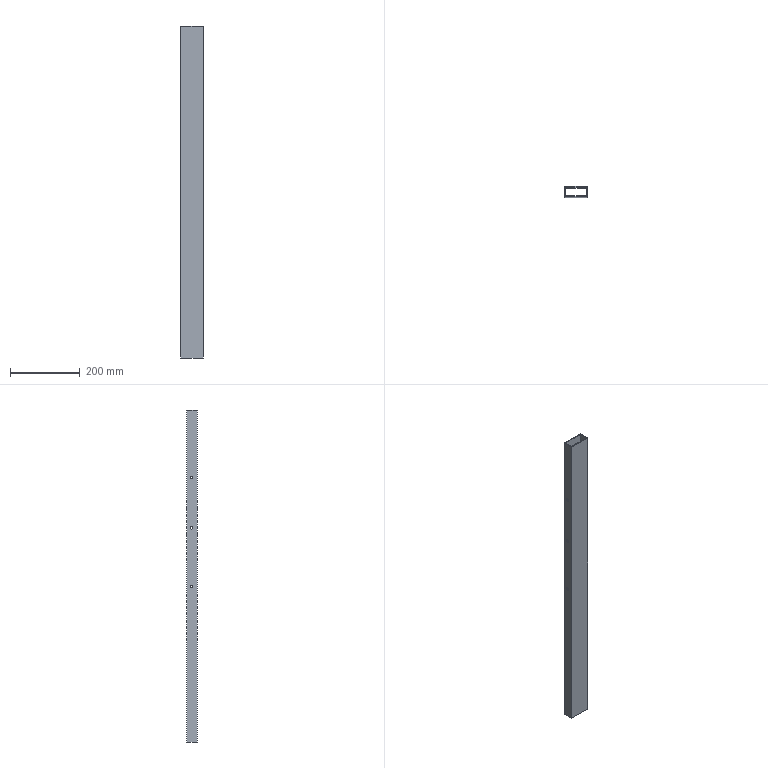Part | SolidWorks | features Cut 1, Extrusion 1, ICE 1 | 1 solid | 22 faces | box 65 x 30 x 950 mm | volume 506395 mm3 | cylinder 12 | plane 10 | commonest cylinder face diameters 8 x12
STEP:
#1=CARTESIAN_POINT('',(24.459,26.308,441.102));
#2=VERTEX_POINT('',#1);
#3=CARTESIAN_POINT('',(24.459,26.308,449.102));
#4=VERTEX_POINT('',#3);
#5=CARTESIAN_POINT('',(24.459,26.308,445.102));
#6=DIRECTION('',(-1.,0.,0.));
#7=DIRECTION('',(0.,0.,1.));
#8=AXIS2_PLACEMENT_3D('',#5,#6,#7);
#9=CIRCLE('',#8,4.);
#10=EDGE_CURVE('',#2,#4,#9,.T.);
#11=ORIENTED_EDGE('',*,*,#10,.F.);
#12=CARTESIAN_POINT('',(21.459,26.308,441.102));
#13=VERTEX_POINT('',#12);
#14=CARTESIAN_POINT('',(24.459,26.308,441.102));
#15=DIRECTION('',(-1.,0.,0.));
#16=VECTOR('',#15,1000.);
#17=LINE('',#14,#16);
#18=EDGE_CURVE('',#2,#13,#17,.T.);
#19=ORIENTED_EDGE('',*,*,#18,.T.);
#20=CARTESIAN_POINT('',(21.459,26.308,449.102));
#21=VERTEX_POINT('',#20);
#22=CARTESIAN_POINT('',(21.459,26.308,445.102));
#23=DIRECTION('',(1.,0.,0.));
#24=DIRECTION('',(0.,1.,0.));
#25=AXIS2_PLACEMENT_3D('',#22,#23,#24);
#26=CIRCLE('',#25,4.);
#27=EDGE_CURVE('',#21,#13,#26,.T.);
#28=ORIENTED_EDGE('',*,*,#27,.F.);
#29=CARTESIAN_POINT('',(24.459,26.308,449.102));
#30=DIRECTION('',(-1.,0.,0.));
#31=VECTOR('',#30,1000.);
#32=LINE('',#29,#31);
#33=EDGE_CURVE('',#4,#21,#32,.T.);
#34=ORIENTED_EDGE('',*,*,#33,.F.);
#35=EDGE_LOOP('',(#11,#19,#28,#34));
#36=FACE_OUTER_BOUND('',#35,.T.);
#37=CARTESIAN_POINT('',(24.459,26.308,445.102));
#38=DIRECTION('',(-1.,0.,0.));
#39=DIRECTION('',(0.,0.,1.));
#40=AXIS2_PLACEMENT_3D('',#37,#38,#39);
#41=CYLINDRICAL_SURFACE('',#40,4.);
#42=ADVANCED_FACE('',(#36),#41,.F.);
#43=CARTESIAN_POINT('',(24.459,26.308,609.102));
#44=VERTEX_POINT('',#43);
#45=CARTESIAN_POINT('',(24.459,26.308,617.102));
#46=VERTEX_POINT('',#45);
#47=CARTESIAN_POINT('',(24.459,26.308,613.102));
#48=DIRECTION('',(-1.,0.,0.));
#49=DIRECTION('',(0.,0.,1.));
#50=AXIS2_PLACEMENT_3D('',#47,#48,#49);
#51=CIRCLE('',#50,4.);
#52=EDGE_CURVE('',#44,#46,#51,.T.);
#53=ORIENTED_EDGE('',*,*,#52,.F.);
#54=CARTESIAN_POINT('',(21.459,26.308,609.102));
#55=VERTEX_POINT('',#54);
#56=CARTESIAN_POINT('',(24.459,26.308,609.102));
#57=DIRECTION('',(-1.,0.,0.));
#58=VECTOR('',#57,1000.);
#59=LINE('',#56,#58);
#60=EDGE_CURVE('',#44,#55,#59,.T.);
#61=ORIENTED_EDGE('',*,*,#60,.T.);
#62=CARTESIAN_POINT('',(21.459,26.308,617.102));
#63=VERTEX_POINT('',#62);
#64=CARTESIAN_POINT('',(21.459,26.308,613.102));
#65=DIRECTION('',(1.,0.,0.));
#66=DIRECTION('',(0.,1.,0.));
#67=AXIS2_PLACEMENT_3D('',#64,#65,#66);
#68=CIRCLE('',#67,4.);
#69=EDGE_CURVE('',#63,#55,#68,.T.);
#70=ORIENTED_EDGE('',*,*,#69,.F.);
#71=CARTESIAN_POINT('',(24.459,26.308,617.102));
#72=DIRECTION('',(-1.,0.,0.));
#73=VECTOR('',#72,1000.);
#74=LINE('',#71,#73);
#75=EDGE_CURVE('',#46,#63,#74,.T.);
#76=ORIENTED_EDGE('',*,*,#75,.F.);
#77=EDGE_LOOP('',(#53,#61,#70,#76));
#78=FACE_OUTER_BOUND('',#77,.T.);
#79=CARTESIAN_POINT('',(24.459,26.308,613.102));
#80=DIRECTION('',(-1.,0.,0.));
#81=DIRECTION('',(0.,0.,1.));
#82=AXIS2_PLACEMENT_3D('',#79,#80,#81);
#83=CYLINDRICAL_SURFACE('',#82,4.);
#84=ADVANCED_FACE('',(#78),#83,.F.);
#85=CARTESIAN_POINT('',(24.459,26.308,753.102));
#86=VERTEX_POINT('',#85);
#87=CARTESIAN_POINT('',(24.459,26.308,761.102));
#88=VERTEX_POINT('',#87);
#89=CARTESIAN_POINT('',(24.459,26.308,757.102));
#90=DIRECTION('',(-1.,0.,0.));
#91=DIRECTION('',(0.,0.,1.));
#92=AXIS2_PLACEMENT_3D('',#89,#90,#91);
#93=CIRCLE('',#92,4.);
#94=EDGE_CURVE('',#86,#88,#93,.T.);
#95=ORIENTED_EDGE('',*,*,#94,.F.);
#96=CARTESIAN_POINT('',(21.459,26.308,753.102));
#97=VERTEX_POINT('',#96);
#98=CARTESIAN_POINT('',(24.459,26.308,753.102));
#99=DIRECTION('',(-1.,0.,0.));
#100=VECTOR('',#99,1000.);
#101=LINE('',#98,#100);
#102=EDGE_CURVE('',#86,#97,#101,.T.);
#103=ORIENTED_EDGE('',*,*,#102,.T.);
#104=CARTESIAN_POINT('',(21.459,26.308,761.102));
#105=VERTEX_POINT('',#104);
#106=CARTESIAN_POINT('',(21.459,26.308,757.102));
#107=DIRECTION('',(1.,0.,0.));
#108=DIRECTION('',(0.,1.,0.));
#109=AXIS2_PLACEMENT_3D('',#106,#107,#108);
#110=CIRCLE('',#109,4.);
#111=EDGE_CURVE('',#105,#97,#110,.T.);
#112=ORIENTED_EDGE('',*,*,#111,.F.);
#113=CARTESIAN_POINT('',(24.459,26.308,761.102));
#114=DIRECTION('',(-1.,0.,0.));
#115=VECTOR('',#114,1000.);
#116=LINE('',#113,#115);
#117=EDGE_CURVE('',#88,#105,#116,.T.);
#118=ORIENTED_EDGE('',*,*,#117,.F.);
#119=EDGE_LOOP('',(#95,#103,#112,#118));
#120=FACE_OUTER_BOUND('',#119,.T.);
#121=CARTESIAN_POINT('',(24.459,26.308,757.102));
#122=DIRECTION('',(-1.,0.,0.));
#123=DIRECTION('',(0.,0.,1.));
#124=AXIS2_PLACEMENT_3D('',#121,#122,#123);
#125=CYLINDRICAL_SURFACE('',#124,4.);
#126=ADVANCED_FACE('',(#120),#125,.F.);
#127=CARTESIAN_POINT('',(-37.541,26.308,441.102));
#128=VERTEX_POINT('',#127);
#129=CARTESIAN_POINT('',(-37.541,26.308,449.102));
#130=VERTEX_POINT('',#129);
#131=CARTESIAN_POINT('',(-37.541,26.308,445.102));
#132=DIRECTION('',(-1.,0.,0.));
#133=DIRECTION('',(0.,0.,1.));
#134=AXIS2_PLACEMENT_3D('',#131,#132,#133);
#135=CIRCLE('',#134,4.);
#136=EDGE_CURVE('',#128,#130,#135,.T.);
#137=ORIENTED_EDGE('',*,*,#136,.F.);
#138=CARTESIAN_POINT('',(-40.541,26.308,441.102));
#139=VERTEX_POINT('',#138);
#140=CARTESIAN_POINT('',(24.459,26.308,441.102));
#141=DIRECTION('',(-1.,0.,0.));
#142=VECTOR('',#141,1000.);
#143=LINE('',#140,#142);
#144=EDGE_CURVE('',#128,#139,#143,.T.);
#145=ORIENTED_EDGE('',*,*,#144,.T.);
#146=CARTESIAN_POINT('',(-40.541,26.308,449.102));
#147=VERTEX_POINT('',#146);
#148=CARTESIAN_POINT('',(-40.541,26.308,445.102));
#149=DIRECTION('',(-1.,0.,0.));
#150=DIRECTION('',(0.,0.,1.));
#151=AXIS2_PLACEMENT_3D('',#148,#149,#150);
#152=CIRCLE('',#151,4.);
#153=EDGE_CURVE('',#139,#147,#152,.T.);
#154=ORIENTED_EDGE('',*,*,#153,.T.);
#155=CARTESIAN_POINT('',(24.459,26.308,449.102));
#156=DIRECTION('',(-1.,0.,0.));
#157=VECTOR('',#156,1000.);
#158=LINE('',#155,#157);
#159=EDGE_CURVE('',#130,#147,#158,.T.);
#160=ORIENTED_EDGE('',*,*,#159,.F.);
#161=EDGE_LOOP('',(#137,#145,#154,#160));
#162=FACE_OUTER_BOUND('',#161,.T.);
#163=CARTESIAN_POINT('',(24.459,26.308,445.102));
#164=DIRECTION('',(-1.,0.,0.));
#165=DIRECTION('',(0.,0.,1.));
#166=AXIS2_PLACEMENT_3D('',#163,#164,#165);
#167=CYLINDRICAL_SURFACE('',#166,4.);
#168=ADVANCED_FACE('',(#162),#167,.F.);
#169=CARTESIAN_POINT('',(-37.541,26.308,609.102));
#170=VERTEX_POINT('',#169);
#171=CARTESIAN_POINT('',(-37.541,26.308,617.102));
#172=VERTEX_POINT('',#171);
#173=CARTESIAN_POINT('',(-37.541,26.308,613.102));
#174=DIRECTION('',(-1.,0.,0.));
#175=DIRECTION('',(0.,0.,1.));
#176=AXIS2_PLACEMENT_3D('',#173,#174,#175);
#177=CIRCLE('',#176,4.);
#178=EDGE_CURVE('',#170,#172,#177,.T.);
#179=ORIENTED_EDGE('',*,*,#178,.F.);
#180=CARTESIAN_POINT('',(-40.541,26.308,609.102));
#181=VERTEX_POINT('',#180);
#182=CARTESIAN_POINT('',(24.459,26.308,609.102));
#183=DIRECTION('',(-1.,0.,0.));
#184=VECTOR('',#183,1000.);
#185=LINE('',#182,#184);
#186=EDGE_CURVE('',#170,#181,#185,.T.);
#187=ORIENTED_EDGE('',*,*,#186,.T.);
#188=CARTESIAN_POINT('',(-40.541,26.308,617.102));
#189=VERTEX_POINT('',#188);
#190=CARTESIAN_POINT('',(-40.541,26.308,613.102));
#191=DIRECTION('',(-1.,0.,0.));
#192=DIRECTION('',(0.,0.,1.));
#193=AXIS2_PLACEMENT_3D('',#190,#191,#192);
#194=CIRCLE('',#193,4.);
#195=EDGE_CURVE('',#181,#189,#194,.T.);
#196=ORIENTED_EDGE('',*,*,#195,.T.);
#197=CARTESIAN_POINT('',(24.459,26.308,617.102));
#198=DIRECTION('',(-1.,0.,0.));
#199=VECTOR('',#198,1000.);
#200=LINE('',#197,#199);
#201=EDGE_CURVE('',#172,#189,#200,.T.);
#202=ORIENTED_EDGE('',*,*,#201,.F.);
#203=EDGE_LOOP('',(#179,#187,#196,#202));
#204=FACE_OUTER_BOUND('',#203,.T.);
#205=CARTESIAN_POINT('',(24.459,26.308,613.102));
#206=DIRECTION('',(-1.,0.,0.));
#207=DIRECTION('',(0.,0.,1.));
#208=AXIS2_PLACEMENT_3D('',#205,#206,#207);
#209=CYLINDRICAL_SURFACE('',#208,4.);
#210=ADVANCED_FACE('',(#204),#209,.F.);
#211=CARTESIAN_POINT('',(-37.541,26.308,753.102));
#212=VERTEX_POINT('',#211);
#213=CARTESIAN_POINT('',(-37.541,26.308,761.102));
#214=VERTEX_POINT('',#213);
#215=CARTESIAN_POINT('',(-37.541,26.308,757.102));
#216=DIRECTION('',(-1.,0.,0.));
#217=DIRECTION('',(0.,0.,1.));
#218=AXIS2_PLACEMENT_3D('',#215,#216,#217);
#219=CIRCLE('',#218,4.);
#220=EDGE_CURVE('',#212,#214,#219,.T.);
#221=ORIENTED_EDGE('',*,*,#220,.F.);
#222=CARTESIAN_POINT('',(-40.541,26.308,753.102));
#223=VERTEX_POINT('',#222);
#224=CARTESIAN_POINT('',(24.459,26.308,753.102));
#225=DIRECTION('',(-1.,0.,0.));
#226=VECTOR('',#225,1000.);
#227=LINE('',#224,#226);
#228=EDGE_CURVE('',#212,#223,#227,.T.);
#229=ORIENTED_EDGE('',*,*,#228,.T.);
#230=CARTESIAN_POINT('',(-40.541,26.308,761.102));
#231=VERTEX_POINT('',#230);
#232=CARTESIAN_POINT('',(-40.541,26.308,757.102));
#233=DIRECTION('',(-1.,0.,0.));
#234=DIRECTION('',(0.,0.,1.));
#235=AXIS2_PLACEMENT_3D('',#232,#233,#234);
#236=CIRCLE('',#235,4.);
#237=EDGE_CURVE('',#223,#231,#236,.T.);
#238=ORIENTED_EDGE('',*,*,#237,.T.);
#239=CARTESIAN_POINT('',(24.459,26.308,761.102));
#240=DIRECTION('',(-1.,0.,0.));
#241=VECTOR('',#240,1000.);
#242=LINE('',#239,#241);
#243=EDGE_CURVE('',#214,#231,#242,.T.);
#244=ORIENTED_EDGE('',*,*,#243,.F.);
#245=EDGE_LOOP('',(#221,#229,#238,#244));
#246=FACE_OUTER_BOUND('',#245,.T.);
#247=CARTESIAN_POINT('',(24.459,26.308,757.102));
#248=DIRECTION('',(-1.,0.,0.));
#249=DIRECTION('',(0.,0.,1.));
#250=AXIS2_PLACEMENT_3D('',#247,#248,#249);
#251=CYLINDRICAL_SURFACE('',#250,4.);
#252=ADVANCED_FACE('',(#246),#251,.F.);
#253=CARTESIAN_POINT('',(-40.541,26.308,445.102));
#254=DIRECTION('',(-1.,0.,0.));
#255=DIRECTION('',(0.,0.,1.));
#256=AXIS2_PLACEMENT_3D('',#253,#254,#255);
#257=CIRCLE('',#256,4.);
#258=EDGE_CURVE('',#147,#139,#257,.T.);
#259=ORIENTED_EDGE('',*,*,#258,.F.);
#260=ORIENTED_EDGE('',*,*,#153,.F.);
#261=EDGE_LOOP('',(#259,#260));
#262=FACE_BOUND('',#261,.T.);
#263=CARTESIAN_POINT('',(-40.541,26.308,613.102));
#264=DIRECTION('',(-1.,0.,0.));
#265=DIRECTION('',(0.,0.,1.));
#266=AXIS2_PLACEMENT_3D('',#263,#264,#265);
#267=CIRCLE('',#266,4.);
#268=EDGE_CURVE('',#189,#181,#267,.T.);
#269=ORIENTED_EDGE('',*,*,#268,.F.);
#270=ORIENTED_EDGE('',*,*,#195,.F.);
#271=EDGE_LOOP('',(#269,#270));
#272=FACE_BOUND('',#271,.T.);
#273=CARTESIAN_POINT('',(-40.541,26.308,757.102));
#274=DIRECTION('',(-1.,0.,0.));
#275=DIRECTION('',(0.,0.,1.));
#276=AXIS2_PLACEMENT_3D('',#273,#274,#275);
#277=CIRCLE('',#276,4.);
#278=EDGE_CURVE('',#231,#223,#277,.T.);
#279=ORIENTED_EDGE('',*,*,#278,.F.);
#280=ORIENTED_EDGE('',*,*,#237,.F.);
#281=EDGE_LOOP('',(#279,#280));
#282=FACE_BOUND('',#281,.T.);
#283=CARTESIAN_POINT('',(-40.541,39.808,0.));
#284=VERTEX_POINT('',#283);
#285=CARTESIAN_POINT('',(-40.541,9.808,0.));
#286=VERTEX_POINT('',#285);
#287=CARTESIAN_POINT('',(-40.541,9.808,0.));
#288=DIRECTION('',(0.,-1.,0.));
#289=VECTOR('',#288,1000.);
#290=LINE('',#287,#289);
#291=EDGE_CURVE('',#284,#286,#290,.T.);
#292=ORIENTED_EDGE('',*,*,#291,.T.);
#293=CARTESIAN_POINT('',(-40.541,9.808,950.));
#294=VERTEX_POINT('',#293);
#295=CARTESIAN_POINT('',(-40.541,9.808,950.));
#296=DIRECTION('',(0.,0.,-1.));
#297=VECTOR('',#296,1000.);
#298=LINE('',#295,#297);
#299=EDGE_CURVE('',#294,#286,#298,.T.);
#300=ORIENTED_EDGE('',*,*,#299,.F.);
#301=CARTESIAN_POINT('',(-40.541,39.808,950.));
#302=VERTEX_POINT('',#301);
#303=CARTESIAN_POINT('',(-40.541,9.808,950.));
#304=DIRECTION('',(0.,-1.,0.));
#305=VECTOR('',#304,1000.);
#306=LINE('',#303,#305);
#307=EDGE_CURVE('',#302,#294,#306,.T.);
#308=ORIENTED_EDGE('',*,*,#307,.F.);
#309=CARTESIAN_POINT('',(-40.541,39.808,950.));
#310=DIRECTION('',(0.,0.,-1.));
#311=VECTOR('',#310,1000.);
#312=LINE('',#309,#311);
#313=EDGE_CURVE('',#302,#284,#312,.T.);
#314=ORIENTED_EDGE('',*,*,#313,.T.);
#315=EDGE_LOOP('',(#292,#300,#308,#314));
#316=FACE_OUTER_BOUND('',#315,.T.);
#317=CARTESIAN_POINT('',(-40.541,9.808,950.));
#318=DIRECTION('',(1.,0.,0.));
#319=DIRECTION('',(0.,0.,-1.));
#320=AXIS2_PLACEMENT_3D('',#317,#318,#319);
#321=PLANE('',#320);
#322=ADVANCED_FACE('',(#262,#272,#282,#316),#321,.F.);
#323=CARTESIAN_POINT('',(24.459,9.808,0.));
#324=VERTEX_POINT('',#323);
#325=CARTESIAN_POINT('',(24.459,9.808,0.));
#326=DIRECTION('',(1.,0.,0.));
#327=VECTOR('',#326,1000.);
#328=LINE('',#325,#327);
#329=EDGE_CURVE('',#286,#324,#328,.T.);
#330=ORIENTED_EDGE('',*,*,#329,.T.);
#331=CARTESIAN_POINT('',(24.459,9.808,950.));
#332=VERTEX_POINT('',#331);
#333=CARTESIAN_POINT('',(24.459,9.808,950.));
#334=DIRECTION('',(0.,0.,-1.));
#335=VECTOR('',#334,1000.);
#336=LINE('',#333,#335);
#337=EDGE_CURVE('',#332,#324,#336,.T.);
#338=ORIENTED_EDGE('',*,*,#337,.F.);
#339=CARTESIAN_POINT('',(24.459,9.808,950.));
#340=DIRECTION('',(1.,0.,0.));
#341=VECTOR('',#340,1000.);
#342=LINE('',#339,#341);
#343=EDGE_CURVE('',#294,#332,#342,.T.);
#344=ORIENTED_EDGE('',*,*,#343,.F.);
#345=ORIENTED_EDGE('',*,*,#299,.T.);
#346=EDGE_LOOP('',(#330,#338,#344,#345));
#347=FACE_OUTER_BOUND('',#346,.T.);
#348=CARTESIAN_POINT('',(24.459,9.808,950.));
#349=DIRECTION('',(0.,1.,0.));
#350=DIRECTION('',(0.,0.,1.));
#351=AXIS2_PLACEMENT_3D('',#348,#349,#350);
#352=PLANE('',#351);
#353=ADVANCED_FACE('',(#347),#352,.F.);
#354=CARTESIAN_POINT('',(24.459,26.308,445.102));
#355=DIRECTION('',(-1.,0.,0.));
#356=DIRECTION('',(0.,0.,1.));
#357=AXIS2_PLACEMENT_3D('',#354,#355,#356);
#358=CIRCLE('',#357,4.);
#359=EDGE_CURVE('',#4,#2,#358,.T.);
#360=ORIENTED_EDGE('',*,*,#359,.T.);
#361=ORIENTED_EDGE('',*,*,#10,.T.);
#362=EDGE_LOOP('',(#360,#361));
#363=FACE_BOUND('',#362,.T.);
#364=CARTESIAN_POINT('',(24.459,26.308,613.102));
#365=DIRECTION('',(-1.,0.,0.));
#366=DIRECTION('',(0.,0.,1.));
#367=AXIS2_PLACEMENT_3D('',#364,#365,#366);
#368=CIRCLE('',#367,4.);
#369=EDGE_CURVE('',#46,#44,#368,.T.);
#370=ORIENTED_EDGE('',*,*,#369,.T.);
#371=ORIENTED_EDGE('',*,*,#52,.T.);
#372=EDGE_LOOP('',(#370,#371));
#373=FACE_BOUND('',#372,.T.);
#374=CARTESIAN_POINT('',(24.459,26.308,757.102));
#375=DIRECTION('',(-1.,0.,0.));
#376=DIRECTION('',(0.,0.,1.));
#377=AXIS2_PLACEMENT_3D('',#374,#375,#376);
#378=CIRCLE('',#377,4.);
#379=EDGE_CURVE('',#88,#86,#378,.T.);
#380=ORIENTED_EDGE('',*,*,#379,.T.);
#381=ORIENTED_EDGE('',*,*,#94,.T.);
#382=EDGE_LOOP('',(#380,#381));
#383=FACE_BOUND('',#382,.T.);
#384=CARTESIAN_POINT('',(24.459,39.808,0.));
#385=VERTEX_POINT('',#384);
#386=CARTESIAN_POINT('',(24.459,39.808,0.));
#387=DIRECTION('',(0.,1.,0.));
#388=VECTOR('',#387,1000.);
#389=LINE('',#386,#388);
#390=EDGE_CURVE('',#324,#385,#389,.T.);
#391=ORIENTED_EDGE('',*,*,#390,.T.);
#392=CARTESIAN_POINT('',(24.459,39.808,950.));
#393=VERTEX_POINT('',#392);
#394=CARTESIAN_POINT('',(24.459,39.808,950.));
#395=DIRECTION('',(0.,0.,-1.));
#396=VECTOR('',#395,1000.);
#397=LINE('',#394,#396);
#398=EDGE_CURVE('',#393,#385,#397,.T.);
#399=ORIENTED_EDGE('',*,*,#398,.F.);
#400=CARTESIAN_POINT('',(24.459,39.808,950.));
#401=DIRECTION('',(0.,1.,0.));
#402=VECTOR('',#401,1000.);
#403=LINE('',#400,#402);
#404=EDGE_CURVE('',#332,#393,#403,.T.);
#405=ORIENTED_EDGE('',*,*,#404,.F.);
#406=ORIENTED_EDGE('',*,*,#337,.T.);
#407=EDGE_LOOP('',(#391,#399,#405,#406));
#408=FACE_OUTER_BOUND('',#407,.T.);
#409=CARTESIAN_POINT('',(24.459,39.808,950.));
#410=DIRECTION('',(-1.,0.,0.));
#411=DIRECTION('',(0.,0.,1.));
#412=AXIS2_PLACEMENT_3D('',#409,#410,#411);
#413=PLANE('',#412);
#414=ADVANCED_FACE('',(#363,#373,#383,#408),#413,.F.);
#415=CARTESIAN_POINT('',(-40.541,39.808,0.));
#416=DIRECTION('',(-1.,0.,0.));
#417=VECTOR('',#416,1000.);
#418=LINE('',#415,#417);
#419=EDGE_CURVE('',#385,#284,#418,.T.);
#420=ORIENTED_EDGE('',*,*,#419,.T.);
#421=ORIENTED_EDGE('',*,*,#313,.F.);
#422=CARTESIAN_POINT('',(-40.541,39.808,950.));
#423=DIRECTION('',(-1.,0.,0.));
#424=VECTOR('',#423,1000.);
#425=LINE('',#422,#424);
#426=EDGE_CURVE('',#393,#302,#425,.T.);
#427=ORIENTED_EDGE('',*,*,#426,.F.);
#428=ORIENTED_EDGE('',*,*,#398,.T.);
#429=EDGE_LOOP('',(#420,#421,#427,#428));
#430=FACE_OUTER_BOUND('',#429,.T.);
#431=CARTESIAN_POINT('',(-40.541,39.808,950.));
#432=DIRECTION('',(0.,-1.,0.));
#433=DIRECTION('',(0.,0.,-1.));
#434=AXIS2_PLACEMENT_3D('',#431,#432,#433);
#435=PLANE('',#434);
#436=ADVANCED_FACE('',(#430),#435,.F.);
#437=CARTESIAN_POINT('',(21.459,36.808,950.));
#438=VERTEX_POINT('',#437);
#439=CARTESIAN_POINT('',(-37.541,36.808,950.));
#440=VERTEX_POINT('',#439);
#441=CARTESIAN_POINT('',(-37.541,36.808,950.));
#442=DIRECTION('',(-1.,0.,0.));
#443=VECTOR('',#442,1000.);
#444=LINE('',#441,#443);
#445=EDGE_CURVE('',#438,#440,#444,.T.);
#446=ORIENTED_EDGE('',*,*,#445,.F.);
#447=CARTESIAN_POINT('',(21.459,12.808,950.));
#448=VERTEX_POINT('',#447);
#449=CARTESIAN_POINT('',(21.459,36.808,950.));
#450=DIRECTION('',(0.,1.,0.));
#451=VECTOR('',#450,1000.);
#452=LINE('',#449,#451);
#453=EDGE_CURVE('',#448,#438,#452,.T.);
#454=ORIENTED_EDGE('',*,*,#453,.F.);
#455=CARTESIAN_POINT('',(-37.541,12.808,950.));
#456=VERTEX_POINT('',#455);
#457=CARTESIAN_POINT('',(21.459,12.808,950.));
#458=DIRECTION('',(1.,0.,0.));
#459=VECTOR('',#458,1000.);
#460=LINE('',#457,#459);
#461=EDGE_CURVE('',#456,#448,#460,.T.);
#462=ORIENTED_EDGE('',*,*,#461,.F.);
#463=CARTESIAN_POINT('',(-37.541,12.808,950.));
#464=DIRECTION('',(0.,-1.,0.));
#465=VECTOR('',#464,1000.);
#466=LINE('',#463,#465);
#467=EDGE_CURVE('',#440,#456,#466,.T.);
#468=ORIENTED_EDGE('',*,*,#467,.F.);
#469=EDGE_LOOP('',(#446,#454,#462,#468));
#470=FACE_BOUND('',#469,.T.);
#471=ORIENTED_EDGE('',*,*,#307,.T.);
#472=ORIENTED_EDGE('',*,*,#343,.T.);
#473=ORIENTED_EDGE('',*,*,#404,.T.);
#474=ORIENTED_EDGE('',*,*,#426,.T.);
#475=EDGE_LOOP('',(#471,#472,#473,#474));
#476=FACE_OUTER_BOUND('',#475,.T.);
#477=CARTESIAN_POINT('',(0.,0.,950.));
#478=DIRECTION('',(0.,0.,-1.));
#479=DIRECTION('',(-1.,0.,0.));
#480=AXIS2_PLACEMENT_3D('',#477,#478,#479);
#481=PLANE('',#480);
#482=ADVANCED_FACE('',(#470,#476),#481,.F.);
#483=CARTESIAN_POINT('',(21.459,12.808,0.));
#484=VERTEX_POINT('',#483);
#485=CARTESIAN_POINT('',(21.459,36.808,0.));
#486=VERTEX_POINT('',#485);
#487=CARTESIAN_POINT('',(21.459,36.808,0.));
#488=DIRECTION('',(0.,1.,0.));
#489=VECTOR('',#488,1000.);
#490=LINE('',#487,#489);
#491=EDGE_CURVE('',#484,#486,#490,.T.);
#492=ORIENTED_EDGE('',*,*,#491,.T.);
#493=CARTESIAN_POINT('',(-37.541,36.808,0.));
#494=VERTEX_POINT('',#493);
#495=CARTESIAN_POINT('',(-37.541,36.808,0.));
#496=DIRECTION('',(-1.,0.,0.));
#497=VECTOR('',#496,1000.);
#498=LINE('',#495,#497);
#499=EDGE_CURVE('',#486,#494,#498,.T.);
#500=ORIENTED_EDGE('',*,*,#499,.T.);
#501=CARTESIAN_POINT('',(-37.541,12.808,0.));
#502=VERTEX_POINT('',#501);
#503=CARTESIAN_POINT('',(-37.541,12.808,0.));
#504=DIRECTION('',(0.,-1.,0.));
#505=VECTOR('',#504,1000.);
#506=LINE('',#503,#505);
#507=EDGE_CURVE('',#494,#502,#506,.T.);
#508=ORIENTED_EDGE('',*,*,#507,.T.);
#509=CARTESIAN_POINT('',(21.459,12.808,0.));
#510=DIRECTION('',(1.,0.,0.));
#511=VECTOR('',#510,1000.);
#512=LINE('',#509,#511);
#513=EDGE_CURVE('',#502,#484,#512,.T.);
#514=ORIENTED_EDGE('',*,*,#513,.T.);
#515=EDGE_LOOP('',(#492,#500,#508,#514));
#516=FACE_BOUND('',#515,.T.);
#517=ORIENTED_EDGE('',*,*,#291,.F.);
#518=ORIENTED_EDGE('',*,*,#419,.F.);
#519=ORIENTED_EDGE('',*,*,#390,.F.);
#520=ORIENTED_EDGE('',*,*,#329,.F.);
#521=EDGE_LOOP('',(#517,#518,#519,#520));
#522=FACE_OUTER_BOUND('',#521,.T.);
#523=CARTESIAN_POINT('',(0.,0.,0.));
#524=DIRECTION('',(0.,0.,-1.));
#525=DIRECTION('',(-1.,0.,0.));
#526=AXIS2_PLACEMENT_3D('',#523,#524,#525);
#527=PLANE('',#526);
#528=ADVANCED_FACE('',(#516,#522),#527,.T.);
#529=ORIENTED_EDGE('',*,*,#27,.T.);
#530=CARTESIAN_POINT('',(21.459,26.308,445.102));
#531=DIRECTION('',(1.,0.,0.));
#532=DIRECTION('',(0.,1.,0.));
#533=AXIS2_PLACEMENT_3D('',#530,#531,#532);
#534=CIRCLE('',#533,4.);
#535=EDGE_CURVE('',#13,#21,#534,.T.);
#536=ORIENTED_EDGE('',*,*,#535,.T.);
#537=EDGE_LOOP('',(#529,#536));
#538=FACE_BOUND('',#537,.T.);
#539=ORIENTED_EDGE('',*,*,#69,.T.);
#540=CARTESIAN_POINT('',(21.459,26.308,613.102));
#541=DIRECTION('',(1.,0.,0.));
#542=DIRECTION('',(0.,1.,0.));
#543=AXIS2_PLACEMENT_3D('',#540,#541,#542);
#544=CIRCLE('',#543,4.);
#545=EDGE_CURVE('',#55,#63,#544,.T.);
#546=ORIENTED_EDGE('',*,*,#545,.T.);
#547=EDGE_LOOP('',(#539,#546));
#548=FACE_BOUND('',#547,.T.);
#549=ORIENTED_EDGE('',*,*,#111,.T.);
#550=CARTESIAN_POINT('',(21.459,26.308,757.102));
#551=DIRECTION('',(1.,0.,0.));
#552=DIRECTION('',(0.,1.,0.));
#553=AXIS2_PLACEMENT_3D('',#550,#551,#552);
#554=CIRCLE('',#553,4.);
#555=EDGE_CURVE('',#97,#105,#554,.T.);
#556=ORIENTED_EDGE('',*,*,#555,.T.);
#557=EDGE_LOOP('',(#549,#556));
#558=FACE_BOUND('',#557,.T.);
#559=ORIENTED_EDGE('',*,*,#453,.T.);
#560=CARTESIAN_POINT('',(21.459,36.808,0.));
#561=DIRECTION('',(0.,0.,1.));
#562=VECTOR('',#561,1000.);
#563=LINE('',#560,#562);
#564=EDGE_CURVE('',#486,#438,#563,.T.);
#565=ORIENTED_EDGE('',*,*,#564,.F.);
#566=ORIENTED_EDGE('',*,*,#491,.F.);
#567=CARTESIAN_POINT('',(21.459,12.808,0.));
#568=DIRECTION('',(0.,0.,1.));
#569=VECTOR('',#568,1000.);
#570=LINE('',#567,#569);
#571=EDGE_CURVE('',#484,#448,#570,.T.);
#572=ORIENTED_EDGE('',*,*,#571,.T.);
#573=EDGE_LOOP('',(#559,#565,#566,#572));
#574=FACE_OUTER_BOUND('',#573,.T.);
#575=CARTESIAN_POINT('',(21.459,36.808,0.));
#576=DIRECTION('',(1.,0.,0.));
#577=DIRECTION('',(0.,1.,0.));
#578=AXIS2_PLACEMENT_3D('',#575,#576,#577);
#579=PLANE('',#578);
#580=ADVANCED_FACE('',(#538,#548,#558,#574),#579,.F.);
#581=ORIENTED_EDGE('',*,*,#461,.T.);
#582=ORIENTED_EDGE('',*,*,#571,.F.);
#583=ORIENTED_EDGE('',*,*,#513,.F.);
#584=CARTESIAN_POINT('',(-37.541,12.808,0.));
#585=DIRECTION('',(0.,0.,1.));
#586=VECTOR('',#585,1000.);
#587=LINE('',#584,#586);
#588=EDGE_CURVE('',#502,#456,#587,.T.);
#589=ORIENTED_EDGE('',*,*,#588,.T.);
#590=EDGE_LOOP('',(#581,#582,#583,#589));
#591=FACE_OUTER_BOUND('',#590,.T.);
#592=CARTESIAN_POINT('',(21.459,12.808,0.));
#593=DIRECTION('',(0.,-1.,0.));
#594=DIRECTION('',(1.,0.,0.));
#595=AXIS2_PLACEMENT_3D('',#592,#593,#594);
#596=PLANE('',#595);
#597=ADVANCED_FACE('',(#591),#596,.F.);
#598=CARTESIAN_POINT('',(-37.541,26.308,445.102));
#599=DIRECTION('',(-1.,0.,0.));
#600=DIRECTION('',(0.,0.,1.));
#601=AXIS2_PLACEMENT_3D('',#598,#599,#600);
#602=CIRCLE('',#601,4.);
#603=EDGE_CURVE('',#130,#128,#602,.T.);
#604=ORIENTED_EDGE('',*,*,#603,.T.);
#605=ORIENTED_EDGE('',*,*,#136,.T.);
#606=EDGE_LOOP('',(#604,#605));
#607=FACE_BOUND('',#606,.T.);
#608=CARTESIAN_POINT('',(-37.541,26.308,613.102));
#609=DIRECTION('',(-1.,0.,0.));
#610=DIRECTION('',(0.,0.,1.));
#611=AXIS2_PLACEMENT_3D('',#608,#609,#610);
#612=CIRCLE('',#611,4.);
#613=EDGE_CURVE('',#172,#170,#612,.T.);
#614=ORIENTED_EDGE('',*,*,#613,.T.);
#615=ORIENTED_EDGE('',*,*,#178,.T.);
#616=EDGE_LOOP('',(#614,#615));
#617=FACE_BOUND('',#616,.T.);
#618=CARTESIAN_POINT('',(-37.541,26.308,757.102));
#619=DIRECTION('',(-1.,0.,0.));
#620=DIRECTION('',(0.,0.,1.));
#621=AXIS2_PLACEMENT_3D('',#618,#619,#620);
#622=CIRCLE('',#621,4.);
#623=EDGE_CURVE('',#214,#212,#622,.T.);
#624=ORIENTED_EDGE('',*,*,#623,.T.);
#625=ORIENTED_EDGE('',*,*,#220,.T.);
#626=EDGE_LOOP('',(#624,#625));
#627=FACE_BOUND('',#626,.T.);
#628=ORIENTED_EDGE('',*,*,#467,.T.);
#629=ORIENTED_EDGE('',*,*,#588,.F.);
#630=ORIENTED_EDGE('',*,*,#507,.F.);
#631=CARTESIAN_POINT('',(-37.541,36.808,0.));
#632=DIRECTION('',(0.,0.,1.));
#633=VECTOR('',#632,1000.);
#634=LINE('',#631,#633);
#635=EDGE_CURVE('',#494,#440,#634,.T.);
#636=ORIENTED_EDGE('',*,*,#635,.T.);
#637=EDGE_LOOP('',(#628,#629,#630,#636));
#638=FACE_OUTER_BOUND('',#637,.T.);
#639=CARTESIAN_POINT('',(-37.541,12.808,0.));
#640=DIRECTION('',(-1.,0.,0.));
#641=DIRECTION('',(0.,0.,1.));
#642=AXIS2_PLACEMENT_3D('',#639,#640,#641);
#643=PLANE('',#642);
#644=ADVANCED_FACE('',(#607,#617,#627,#638),#643,.F.);
#645=ORIENTED_EDGE('',*,*,#445,.T.);
#646=ORIENTED_EDGE('',*,*,#635,.F.);
#647=ORIENTED_EDGE('',*,*,#499,.F.);
#648=ORIENTED_EDGE('',*,*,#564,.T.);
#649=EDGE_LOOP('',(#645,#646,#647,#648));
#650=FACE_OUTER_BOUND('',#649,.T.);
#651=CARTESIAN_POINT('',(-37.541,36.808,0.));
#652=DIRECTION('',(0.,1.,0.));
#653=DIRECTION('',(-1.,0.,0.));
#654=AXIS2_PLACEMENT_3D('',#651,#652,#653);
#655=PLANE('',#654);
#656=ADVANCED_FACE('',(#650),#655,.F.);
#657=ORIENTED_EDGE('',*,*,#228,.F.);
#658=ORIENTED_EDGE('',*,*,#623,.F.);
#659=ORIENTED_EDGE('',*,*,#243,.T.);
#660=ORIENTED_EDGE('',*,*,#278,.T.);
#661=EDGE_LOOP('',(#657,#658,#659,#660));
#662=FACE_OUTER_BOUND('',#661,.T.);
#663=CARTESIAN_POINT('',(24.459,26.308,757.102));
#664=DIRECTION('',(-1.,0.,0.));
#665=DIRECTION('',(0.,0.,1.));
#666=AXIS2_PLACEMENT_3D('',#663,#664,#665);
#667=CYLINDRICAL_SURFACE('',#666,4.);
#668=ADVANCED_FACE('',(#662),#667,.F.);
#669=ORIENTED_EDGE('',*,*,#186,.F.);
#670=ORIENTED_EDGE('',*,*,#613,.F.);
#671=ORIENTED_EDGE('',*,*,#201,.T.);
#672=ORIENTED_EDGE('',*,*,#268,.T.);
#673=EDGE_LOOP('',(#669,#670,#671,#672));
#674=FACE_OUTER_BOUND('',#673,.T.);
#675=CARTESIAN_POINT('',(24.459,26.308,613.102));
#676=DIRECTION('',(-1.,0.,0.));
#677=DIRECTION('',(0.,0.,1.));
#678=AXIS2_PLACEMENT_3D('',#675,#676,#677);
#679=CYLINDRICAL_SURFACE('',#678,4.);
#680=ADVANCED_FACE('',(#674),#679,.F.);
#681=ORIENTED_EDGE('',*,*,#144,.F.);
#682=ORIENTED_EDGE('',*,*,#603,.F.);
#683=ORIENTED_EDGE('',*,*,#159,.T.);
#684=ORIENTED_EDGE('',*,*,#258,.T.);
#685=EDGE_LOOP('',(#681,#682,#683,#684));
#686=FACE_OUTER_BOUND('',#685,.T.);
#687=CARTESIAN_POINT('',(24.459,26.308,445.102));
#688=DIRECTION('',(-1.,0.,0.));
#689=DIRECTION('',(0.,0.,1.));
#690=AXIS2_PLACEMENT_3D('',#687,#688,#689);
#691=CYLINDRICAL_SURFACE('',#690,4.);
#692=ADVANCED_FACE('',(#686),#691,.F.);
#693=ORIENTED_EDGE('',*,*,#102,.F.);
#694=ORIENTED_EDGE('',*,*,#379,.F.);
#695=ORIENTED_EDGE('',*,*,#117,.T.);
#696=ORIENTED_EDGE('',*,*,#555,.F.);
#697=EDGE_LOOP('',(#693,#694,#695,#696));
#698=FACE_OUTER_BOUND('',#697,.T.);
#699=CARTESIAN_POINT('',(24.459,26.308,757.102));
#700=DIRECTION('',(-1.,0.,0.));
#701=DIRECTION('',(0.,0.,1.));
#702=AXIS2_PLACEMENT_3D('',#699,#700,#701);
#703=CYLINDRICAL_SURFACE('',#702,4.);
#704=ADVANCED_FACE('',(#698),#703,.F.);
#705=ORIENTED_EDGE('',*,*,#60,.F.);
#706=ORIENTED_EDGE('',*,*,#369,.F.);
#707=ORIENTED_EDGE('',*,*,#75,.T.);
#708=ORIENTED_EDGE('',*,*,#545,.F.);
#709=EDGE_LOOP('',(#705,#706,#707,#708));
#710=FACE_OUTER_BOUND('',#709,.T.);
#711=CARTESIAN_POINT('',(24.459,26.308,613.102));
#712=DIRECTION('',(-1.,0.,0.));
#713=DIRECTION('',(0.,0.,1.));
#714=AXIS2_PLACEMENT_3D('',#711,#712,#713);
#715=CYLINDRICAL_SURFACE('',#714,4.);
#716=ADVANCED_FACE('',(#710),#715,.F.);
#717=ORIENTED_EDGE('',*,*,#18,.F.);
#718=ORIENTED_EDGE('',*,*,#359,.F.);
#719=ORIENTED_EDGE('',*,*,#33,.T.);
#720=ORIENTED_EDGE('',*,*,#535,.F.);
#721=EDGE_LOOP('',(#717,#718,#719,#720));
#722=FACE_OUTER_BOUND('',#721,.T.);
#723=CARTESIAN_POINT('',(24.459,26.308,445.102));
#724=DIRECTION('',(-1.,0.,0.));
#725=DIRECTION('',(0.,0.,1.));
#726=AXIS2_PLACEMENT_3D('',#723,#724,#725);
#727=CYLINDRICAL_SURFACE('',#726,4.);
#728=ADVANCED_FACE('',(#722),#727,.F.);
#729=CLOSED_SHELL('',(#42,#84,#126,#168,#210,#252,#322,#353,#414,#436,#482,#528,#580,#597,#644,#656,#668,#680,#692,#704,#716,#728));
#730=MANIFOLD_SOLID_BREP('',#729);
#731=CARTESIAN_POINT('',(0.,0.,0.));
#732=DIRECTION('',(0.,0.,1.));
#733=DIRECTION('',(1.,0.,0.));
#734=AXIS2_PLACEMENT_3D('',#731,#732,#733);
#735=(LENGTH_UNIT()NAMED_UNIT(*)SI_UNIT(.MILLI.,.METRE.));
#736=UNCERTAINTY_MEASURE_WITH_UNIT(LENGTH_MEASURE(0.00001),#735,'','');
#737=(NAMED_UNIT(*)PLANE_ANGLE_UNIT()SI_UNIT($,.RADIAN.));
#738=(NAMED_UNIT(*)SI_UNIT($,.STERADIAN.)SOLID_ANGLE_UNIT());
#739=(GEOMETRIC_REPRESENTATION_CONTEXT(3)GLOBAL_UNCERTAINTY_ASSIGNED_CONTEXT((#736))GLOBAL_UNIT_ASSIGNED_CONTEXT((#735,#737,#738))REPRESENTATION_CONTEXT('',''));
#740=ADVANCED_BREP_SHAPE_REPRESENTATION('',(#730,#734),#739);